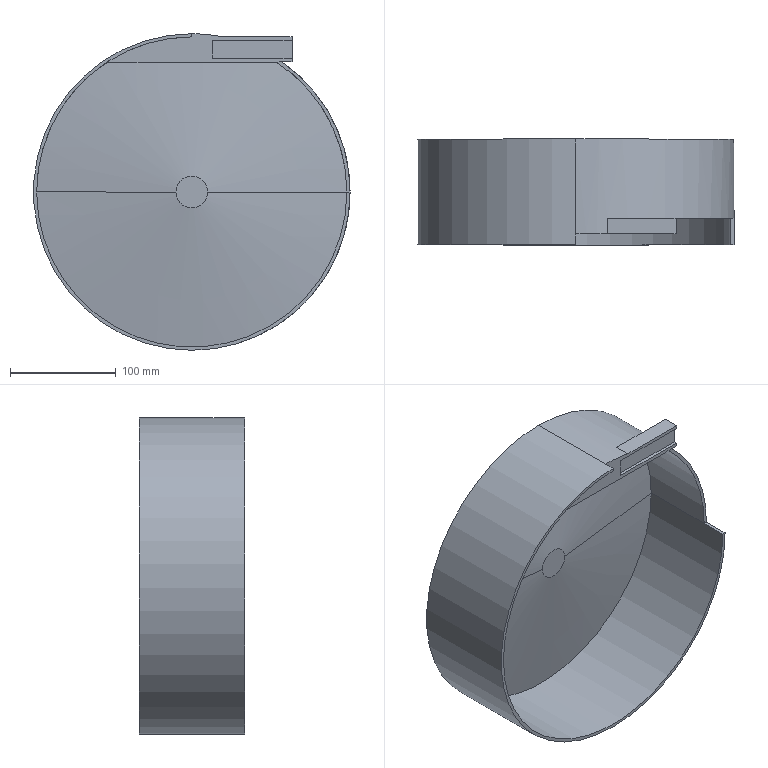Part | STEP file | Vibration plate 20501 | 1 solid | 24 faces | box 300 x 100 x 300 mm | volume 987568 mm3 | plane 18 | cylinder 4 | cone 2 | commonest cylinder face diameters 294 x2 300 x2